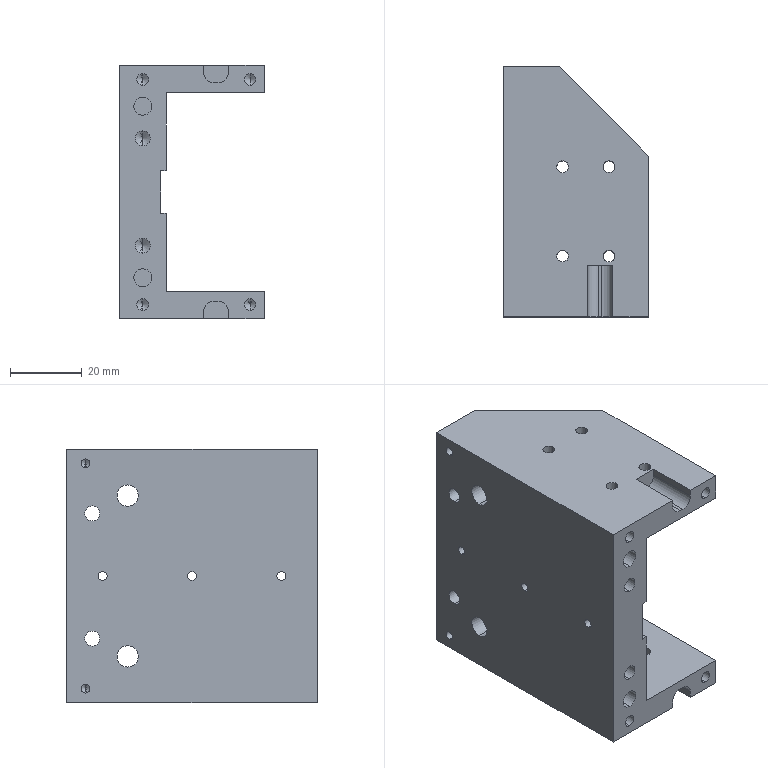Part | STEP file | 11-FG-B02111 | 1 solid | 96 faces | box 40.5 x 70 x 71 mm | volume 84307 mm3 | cylinder 54 | plane 26 | cone 16 | commonest cylinder face diameters 3.3 x24 2.5 x10 4.2 x8 6 x8 5 x4